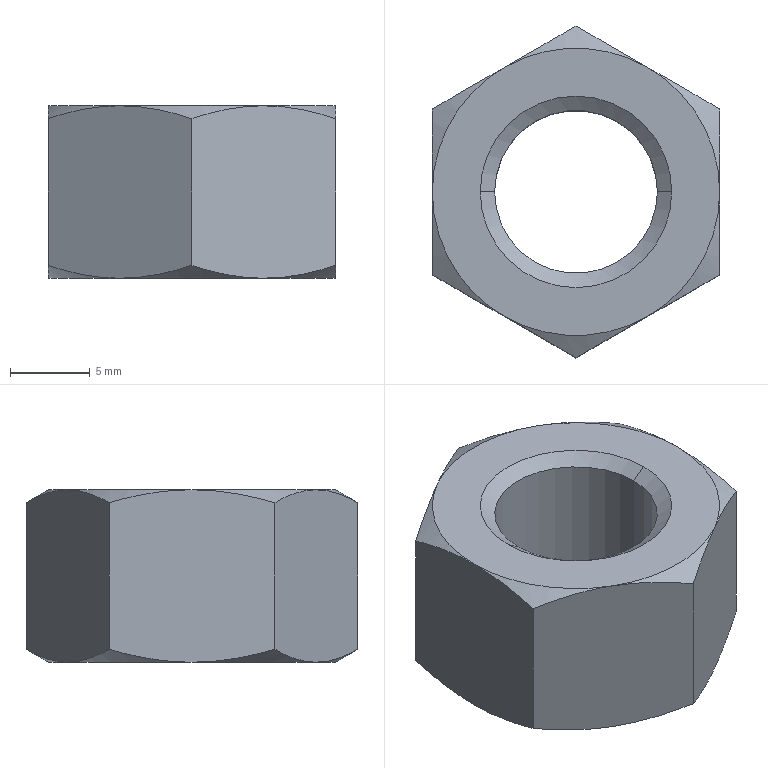Part | STEP file | hex nut style 1_am_B18.2.4.1M - Hex nut, Style 1,  M12 x 1.75 --D-N | 1 solid | 28 faces | box 18 x 20.785 x 10.8 mm | volume 2115 mm3 | cone 16 | plane 8 | cylinder 4 | commonest cylinder face diameters 10.2 x2 12 x2